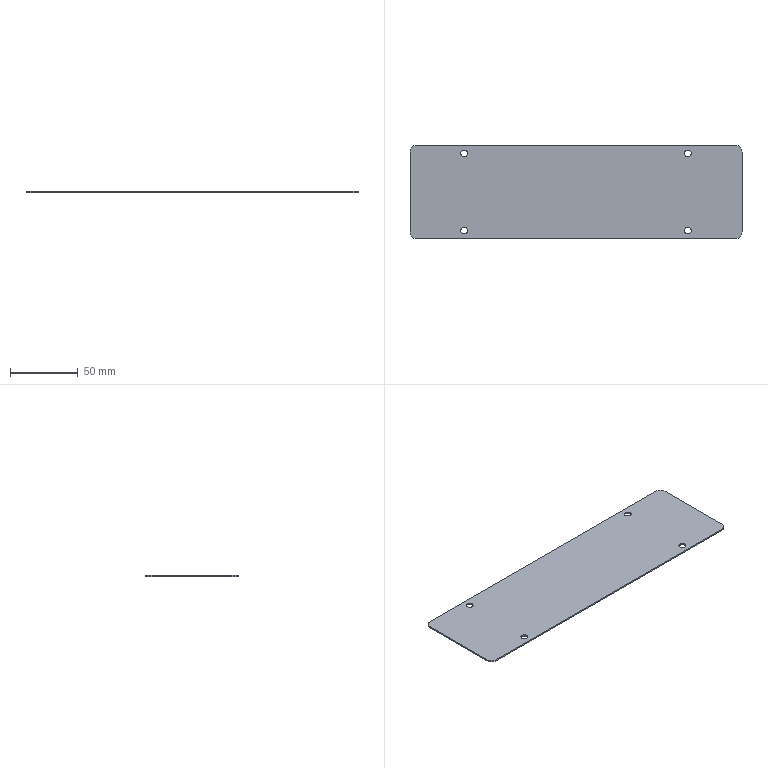Part | SolidWorks | features BaseBody 1 | 1 solid | 18 faces | box 245 x 69 x 1 mm | volume 16805 mm3 | cylinder 12 | plane 6 | commonest cylinder face diameters 5 x8 10 x4
STEP:
#1=CARTESIAN_POINT('',(-85.,-28.5,1.));
#2=VERTEX_POINT('',#1);
#3=CARTESIAN_POINT('',(-80.,-28.5,1.));
#4=VERTEX_POINT('',#3);
#5=CARTESIAN_POINT('',(-82.5,-28.5,1.));
#6=DIRECTION('',(0.,0.,1.));
#7=DIRECTION('',(-1.,0.,0.));
#8=AXIS2_PLACEMENT_3D('',#5,#6,#7);
#9=CIRCLE('',#8,2.5);
#10=EDGE_CURVE('',#2,#4,#9,.T.);
#11=ORIENTED_EDGE('',*,*,#10,.T.);
#12=CARTESIAN_POINT('',(-80.,-28.5,0.));
#13=VERTEX_POINT('',#12);
#14=CARTESIAN_POINT('',(-80.,-28.5,1.));
#15=DIRECTION('',(0.,0.,-1.));
#16=VECTOR('',#15,1000.);
#17=LINE('',#14,#16);
#18=EDGE_CURVE('',#4,#13,#17,.T.);
#19=ORIENTED_EDGE('',*,*,#18,.T.);
#20=CARTESIAN_POINT('',(-85.,-28.5,0.));
#21=VERTEX_POINT('',#20);
#22=CARTESIAN_POINT('',(-82.5,-28.5,0.));
#23=DIRECTION('',(0.,0.,1.));
#24=DIRECTION('',(-1.,0.,0.));
#25=AXIS2_PLACEMENT_3D('',#22,#23,#24);
#26=CIRCLE('',#25,2.5);
#27=EDGE_CURVE('',#21,#13,#26,.T.);
#28=ORIENTED_EDGE('',*,*,#27,.F.);
#29=CARTESIAN_POINT('',(-85.,-28.5,1.));
#30=DIRECTION('',(0.,0.,-1.));
#31=VECTOR('',#30,1000.);
#32=LINE('',#29,#31);
#33=EDGE_CURVE('',#2,#21,#32,.T.);
#34=ORIENTED_EDGE('',*,*,#33,.F.);
#35=EDGE_LOOP('',(#11,#19,#28,#34));
#36=FACE_OUTER_BOUND('',#35,.T.);
#37=CARTESIAN_POINT('',(-82.5,-28.5,1.));
#38=DIRECTION('',(0.,0.,-1.));
#39=DIRECTION('',(-1.,0.,0.));
#40=AXIS2_PLACEMENT_3D('',#37,#38,#39);
#41=CYLINDRICAL_SURFACE('',#40,2.5);
#42=ADVANCED_FACE('',(#36),#41,.F.);
#43=CARTESIAN_POINT('',(80.,-28.5,1.));
#44=VERTEX_POINT('',#43);
#45=CARTESIAN_POINT('',(85.,-28.5,1.));
#46=VERTEX_POINT('',#45);
#47=CARTESIAN_POINT('',(82.5,-28.5,1.));
#48=DIRECTION('',(0.,0.,1.));
#49=DIRECTION('',(-1.,0.,0.));
#50=AXIS2_PLACEMENT_3D('',#47,#48,#49);
#51=CIRCLE('',#50,2.5);
#52=EDGE_CURVE('',#44,#46,#51,.T.);
#53=ORIENTED_EDGE('',*,*,#52,.T.);
#54=CARTESIAN_POINT('',(85.,-28.5,0.));
#55=VERTEX_POINT('',#54);
#56=CARTESIAN_POINT('',(85.,-28.5,1.));
#57=DIRECTION('',(0.,0.,-1.));
#58=VECTOR('',#57,1000.);
#59=LINE('',#56,#58);
#60=EDGE_CURVE('',#46,#55,#59,.T.);
#61=ORIENTED_EDGE('',*,*,#60,.T.);
#62=CARTESIAN_POINT('',(80.,-28.5,0.));
#63=VERTEX_POINT('',#62);
#64=CARTESIAN_POINT('',(82.5,-28.5,0.));
#65=DIRECTION('',(0.,0.,1.));
#66=DIRECTION('',(-1.,0.,0.));
#67=AXIS2_PLACEMENT_3D('',#64,#65,#66);
#68=CIRCLE('',#67,2.5);
#69=EDGE_CURVE('',#63,#55,#68,.T.);
#70=ORIENTED_EDGE('',*,*,#69,.F.);
#71=CARTESIAN_POINT('',(80.,-28.5,1.));
#72=DIRECTION('',(0.,0.,-1.));
#73=VECTOR('',#72,1000.);
#74=LINE('',#71,#73);
#75=EDGE_CURVE('',#44,#63,#74,.T.);
#76=ORIENTED_EDGE('',*,*,#75,.F.);
#77=EDGE_LOOP('',(#53,#61,#70,#76));
#78=FACE_OUTER_BOUND('',#77,.T.);
#79=CARTESIAN_POINT('',(82.5,-28.5,1.));
#80=DIRECTION('',(0.,0.,-1.));
#81=DIRECTION('',(-1.,0.,0.));
#82=AXIS2_PLACEMENT_3D('',#79,#80,#81);
#83=CYLINDRICAL_SURFACE('',#82,2.5);
#84=ADVANCED_FACE('',(#78),#83,.F.);
#85=CARTESIAN_POINT('',(80.,28.5,1.));
#86=VERTEX_POINT('',#85);
#87=CARTESIAN_POINT('',(85.,28.5,1.));
#88=VERTEX_POINT('',#87);
#89=CARTESIAN_POINT('',(82.5,28.5,1.));
#90=DIRECTION('',(0.,0.,1.));
#91=DIRECTION('',(-1.,0.,0.));
#92=AXIS2_PLACEMENT_3D('',#89,#90,#91);
#93=CIRCLE('',#92,2.5);
#94=EDGE_CURVE('',#86,#88,#93,.T.);
#95=ORIENTED_EDGE('',*,*,#94,.T.);
#96=CARTESIAN_POINT('',(85.,28.5,0.));
#97=VERTEX_POINT('',#96);
#98=CARTESIAN_POINT('',(85.,28.5,1.));
#99=DIRECTION('',(0.,0.,-1.));
#100=VECTOR('',#99,1000.);
#101=LINE('',#98,#100);
#102=EDGE_CURVE('',#88,#97,#101,.T.);
#103=ORIENTED_EDGE('',*,*,#102,.T.);
#104=CARTESIAN_POINT('',(80.,28.5,0.));
#105=VERTEX_POINT('',#104);
#106=CARTESIAN_POINT('',(82.5,28.5,0.));
#107=DIRECTION('',(0.,0.,1.));
#108=DIRECTION('',(-1.,0.,0.));
#109=AXIS2_PLACEMENT_3D('',#106,#107,#108);
#110=CIRCLE('',#109,2.5);
#111=EDGE_CURVE('',#105,#97,#110,.T.);
#112=ORIENTED_EDGE('',*,*,#111,.F.);
#113=CARTESIAN_POINT('',(80.,28.5,1.));
#114=DIRECTION('',(0.,0.,-1.));
#115=VECTOR('',#114,1000.);
#116=LINE('',#113,#115);
#117=EDGE_CURVE('',#86,#105,#116,.T.);
#118=ORIENTED_EDGE('',*,*,#117,.F.);
#119=EDGE_LOOP('',(#95,#103,#112,#118));
#120=FACE_OUTER_BOUND('',#119,.T.);
#121=CARTESIAN_POINT('',(82.5,28.5,1.));
#122=DIRECTION('',(0.,0.,-1.));
#123=DIRECTION('',(-1.,0.,0.));
#124=AXIS2_PLACEMENT_3D('',#121,#122,#123);
#125=CYLINDRICAL_SURFACE('',#124,2.5);
#126=ADVANCED_FACE('',(#120),#125,.F.);
#127=CARTESIAN_POINT('',(-85.,28.5,1.));
#128=VERTEX_POINT('',#127);
#129=CARTESIAN_POINT('',(-80.,28.5,1.));
#130=VERTEX_POINT('',#129);
#131=CARTESIAN_POINT('',(-82.5,28.5,1.));
#132=DIRECTION('',(0.,0.,1.));
#133=DIRECTION('',(-1.,0.,0.));
#134=AXIS2_PLACEMENT_3D('',#131,#132,#133);
#135=CIRCLE('',#134,2.5);
#136=EDGE_CURVE('',#128,#130,#135,.T.);
#137=ORIENTED_EDGE('',*,*,#136,.T.);
#138=CARTESIAN_POINT('',(-80.,28.5,0.));
#139=VERTEX_POINT('',#138);
#140=CARTESIAN_POINT('',(-80.,28.5,1.));
#141=DIRECTION('',(0.,0.,-1.));
#142=VECTOR('',#141,1000.);
#143=LINE('',#140,#142);
#144=EDGE_CURVE('',#130,#139,#143,.T.);
#145=ORIENTED_EDGE('',*,*,#144,.T.);
#146=CARTESIAN_POINT('',(-85.,28.5,0.));
#147=VERTEX_POINT('',#146);
#148=CARTESIAN_POINT('',(-82.5,28.5,0.));
#149=DIRECTION('',(0.,0.,1.));
#150=DIRECTION('',(-1.,0.,0.));
#151=AXIS2_PLACEMENT_3D('',#148,#149,#150);
#152=CIRCLE('',#151,2.5);
#153=EDGE_CURVE('',#147,#139,#152,.T.);
#154=ORIENTED_EDGE('',*,*,#153,.F.);
#155=CARTESIAN_POINT('',(-85.,28.5,1.));
#156=DIRECTION('',(0.,0.,-1.));
#157=VECTOR('',#156,1000.);
#158=LINE('',#155,#157);
#159=EDGE_CURVE('',#128,#147,#158,.T.);
#160=ORIENTED_EDGE('',*,*,#159,.F.);
#161=EDGE_LOOP('',(#137,#145,#154,#160));
#162=FACE_OUTER_BOUND('',#161,.T.);
#163=CARTESIAN_POINT('',(-82.5,28.5,1.));
#164=DIRECTION('',(0.,0.,-1.));
#165=DIRECTION('',(-1.,0.,0.));
#166=AXIS2_PLACEMENT_3D('',#163,#164,#165);
#167=CYLINDRICAL_SURFACE('',#166,2.5);
#168=ADVANCED_FACE('',(#162),#167,.F.);
#169=ORIENTED_EDGE('',*,*,#10,.F.);
#170=CARTESIAN_POINT('',(-82.5,-28.5,1.));
#171=DIRECTION('',(0.,0.,1.));
#172=DIRECTION('',(-1.,0.,0.));
#173=AXIS2_PLACEMENT_3D('',#170,#171,#172);
#174=CIRCLE('',#173,2.5);
#175=EDGE_CURVE('',#4,#2,#174,.T.);
#176=ORIENTED_EDGE('',*,*,#175,.F.);
#177=EDGE_LOOP('',(#169,#176));
#178=FACE_BOUND('',#177,.T.);
#179=ORIENTED_EDGE('',*,*,#52,.F.);
#180=CARTESIAN_POINT('',(82.5,-28.5,1.));
#181=DIRECTION('',(0.,0.,1.));
#182=DIRECTION('',(-1.,0.,0.));
#183=AXIS2_PLACEMENT_3D('',#180,#181,#182);
#184=CIRCLE('',#183,2.5);
#185=EDGE_CURVE('',#46,#44,#184,.T.);
#186=ORIENTED_EDGE('',*,*,#185,.F.);
#187=EDGE_LOOP('',(#179,#186));
#188=FACE_BOUND('',#187,.T.);
#189=ORIENTED_EDGE('',*,*,#94,.F.);
#190=CARTESIAN_POINT('',(82.5,28.5,1.));
#191=DIRECTION('',(0.,0.,1.));
#192=DIRECTION('',(-1.,0.,0.));
#193=AXIS2_PLACEMENT_3D('',#190,#191,#192);
#194=CIRCLE('',#193,2.5);
#195=EDGE_CURVE('',#88,#86,#194,.T.);
#196=ORIENTED_EDGE('',*,*,#195,.F.);
#197=EDGE_LOOP('',(#189,#196));
#198=FACE_BOUND('',#197,.T.);
#199=ORIENTED_EDGE('',*,*,#136,.F.);
#200=CARTESIAN_POINT('',(-82.5,28.5,1.));
#201=DIRECTION('',(0.,0.,1.));
#202=DIRECTION('',(-1.,0.,0.));
#203=AXIS2_PLACEMENT_3D('',#200,#201,#202);
#204=CIRCLE('',#203,2.5);
#205=EDGE_CURVE('',#130,#128,#204,.T.);
#206=ORIENTED_EDGE('',*,*,#205,.F.);
#207=EDGE_LOOP('',(#199,#206));
#208=FACE_BOUND('',#207,.T.);
#209=CARTESIAN_POINT('',(117.5,-34.5,1.));
#210=VERTEX_POINT('',#209);
#211=CARTESIAN_POINT('',(-117.5,-34.5,1.));
#212=VERTEX_POINT('',#211);
#213=CARTESIAN_POINT('',(-117.5,-34.5,1.));
#214=DIRECTION('',(-1.,0.,0.));
#215=VECTOR('',#214,1000.);
#216=LINE('',#213,#215);
#217=EDGE_CURVE('',#210,#212,#216,.T.);
#218=ORIENTED_EDGE('',*,*,#217,.F.);
#219=CARTESIAN_POINT('',(122.5,-29.5,1.));
#220=VERTEX_POINT('',#219);
#221=CARTESIAN_POINT('',(117.5,-29.5,1.));
#222=DIRECTION('',(0.,0.,-1.));
#223=DIRECTION('',(-1.,0.,0.));
#224=AXIS2_PLACEMENT_3D('',#221,#222,#223);
#225=CIRCLE('',#224,5.);
#226=EDGE_CURVE('',#220,#210,#225,.T.);
#227=ORIENTED_EDGE('',*,*,#226,.F.);
#228=CARTESIAN_POINT('',(122.5,29.5,1.));
#229=VERTEX_POINT('',#228);
#230=CARTESIAN_POINT('',(122.5,-29.5,1.));
#231=DIRECTION('',(0.,-1.,0.));
#232=VECTOR('',#231,1000.);
#233=LINE('',#230,#232);
#234=EDGE_CURVE('',#229,#220,#233,.T.);
#235=ORIENTED_EDGE('',*,*,#234,.F.);
#236=CARTESIAN_POINT('',(117.5,34.5,1.));
#237=VERTEX_POINT('',#236);
#238=CARTESIAN_POINT('',(117.5,29.5,1.));
#239=DIRECTION('',(0.,0.,-1.));
#240=DIRECTION('',(-1.,0.,0.));
#241=AXIS2_PLACEMENT_3D('',#238,#239,#240);
#242=CIRCLE('',#241,5.);
#243=EDGE_CURVE('',#237,#229,#242,.T.);
#244=ORIENTED_EDGE('',*,*,#243,.F.);
#245=CARTESIAN_POINT('',(-117.5,34.5,1.));
#246=VERTEX_POINT('',#245);
#247=CARTESIAN_POINT('',(-117.5,34.5,1.));
#248=DIRECTION('',(1.,0.,0.));
#249=VECTOR('',#248,1000.);
#250=LINE('',#247,#249);
#251=EDGE_CURVE('',#246,#237,#250,.T.);
#252=ORIENTED_EDGE('',*,*,#251,.F.);
#253=CARTESIAN_POINT('',(-122.5,29.5,1.));
#254=VERTEX_POINT('',#253);
#255=CARTESIAN_POINT('',(-117.5,29.5,1.));
#256=DIRECTION('',(0.,0.,-1.));
#257=DIRECTION('',(-1.,0.,0.));
#258=AXIS2_PLACEMENT_3D('',#255,#256,#257);
#259=CIRCLE('',#258,5.);
#260=EDGE_CURVE('',#254,#246,#259,.T.);
#261=ORIENTED_EDGE('',*,*,#260,.F.);
#262=CARTESIAN_POINT('',(-122.5,-29.5,1.));
#263=VERTEX_POINT('',#262);
#264=CARTESIAN_POINT('',(-122.5,-29.5,1.));
#265=DIRECTION('',(0.,1.,0.));
#266=VECTOR('',#265,1000.);
#267=LINE('',#264,#266);
#268=EDGE_CURVE('',#263,#254,#267,.T.);
#269=ORIENTED_EDGE('',*,*,#268,.F.);
#270=CARTESIAN_POINT('',(-117.5,-29.5,1.));
#271=DIRECTION('',(0.,0.,-1.));
#272=DIRECTION('',(-1.,0.,0.));
#273=AXIS2_PLACEMENT_3D('',#270,#271,#272);
#274=CIRCLE('',#273,5.);
#275=EDGE_CURVE('',#212,#263,#274,.T.);
#276=ORIENTED_EDGE('',*,*,#275,.F.);
#277=EDGE_LOOP('',(#218,#227,#235,#244,#252,#261,#269,#276));
#278=FACE_OUTER_BOUND('',#277,.T.);
#279=CARTESIAN_POINT('',(-117.5,-29.5,1.));
#280=DIRECTION('',(0.,0.,-1.));
#281=DIRECTION('',(-1.,0.,0.));
#282=AXIS2_PLACEMENT_3D('',#279,#280,#281);
#283=PLANE('',#282);
#284=ADVANCED_FACE('',(#178,#188,#198,#208,#278),#283,.F.);
#285=ORIENTED_EDGE('',*,*,#18,.F.);
#286=ORIENTED_EDGE('',*,*,#175,.T.);
#287=ORIENTED_EDGE('',*,*,#33,.T.);
#288=CARTESIAN_POINT('',(-82.5,-28.5,0.));
#289=DIRECTION('',(0.,0.,1.));
#290=DIRECTION('',(-1.,0.,0.));
#291=AXIS2_PLACEMENT_3D('',#288,#289,#290);
#292=CIRCLE('',#291,2.5);
#293=EDGE_CURVE('',#13,#21,#292,.T.);
#294=ORIENTED_EDGE('',*,*,#293,.F.);
#295=EDGE_LOOP('',(#285,#286,#287,#294));
#296=FACE_OUTER_BOUND('',#295,.T.);
#297=CARTESIAN_POINT('',(-82.5,-28.5,1.));
#298=DIRECTION('',(0.,0.,-1.));
#299=DIRECTION('',(-1.,0.,0.));
#300=AXIS2_PLACEMENT_3D('',#297,#298,#299);
#301=CYLINDRICAL_SURFACE('',#300,2.5);
#302=ADVANCED_FACE('',(#296),#301,.F.);
#303=ORIENTED_EDGE('',*,*,#60,.F.);
#304=ORIENTED_EDGE('',*,*,#185,.T.);
#305=ORIENTED_EDGE('',*,*,#75,.T.);
#306=CARTESIAN_POINT('',(82.5,-28.5,0.));
#307=DIRECTION('',(0.,0.,1.));
#308=DIRECTION('',(-1.,0.,0.));
#309=AXIS2_PLACEMENT_3D('',#306,#307,#308);
#310=CIRCLE('',#309,2.5);
#311=EDGE_CURVE('',#55,#63,#310,.T.);
#312=ORIENTED_EDGE('',*,*,#311,.F.);
#313=EDGE_LOOP('',(#303,#304,#305,#312));
#314=FACE_OUTER_BOUND('',#313,.T.);
#315=CARTESIAN_POINT('',(82.5,-28.5,1.));
#316=DIRECTION('',(0.,0.,-1.));
#317=DIRECTION('',(-1.,0.,0.));
#318=AXIS2_PLACEMENT_3D('',#315,#316,#317);
#319=CYLINDRICAL_SURFACE('',#318,2.5);
#320=ADVANCED_FACE('',(#314),#319,.F.);
#321=ORIENTED_EDGE('',*,*,#102,.F.);
#322=ORIENTED_EDGE('',*,*,#195,.T.);
#323=ORIENTED_EDGE('',*,*,#117,.T.);
#324=CARTESIAN_POINT('',(82.5,28.5,0.));
#325=DIRECTION('',(0.,0.,1.));
#326=DIRECTION('',(-1.,0.,0.));
#327=AXIS2_PLACEMENT_3D('',#324,#325,#326);
#328=CIRCLE('',#327,2.5);
#329=EDGE_CURVE('',#97,#105,#328,.T.);
#330=ORIENTED_EDGE('',*,*,#329,.F.);
#331=EDGE_LOOP('',(#321,#322,#323,#330));
#332=FACE_OUTER_BOUND('',#331,.T.);
#333=CARTESIAN_POINT('',(82.5,28.5,1.));
#334=DIRECTION('',(0.,0.,-1.));
#335=DIRECTION('',(-1.,0.,0.));
#336=AXIS2_PLACEMENT_3D('',#333,#334,#335);
#337=CYLINDRICAL_SURFACE('',#336,2.5);
#338=ADVANCED_FACE('',(#332),#337,.F.);
#339=ORIENTED_EDGE('',*,*,#144,.F.);
#340=ORIENTED_EDGE('',*,*,#205,.T.);
#341=ORIENTED_EDGE('',*,*,#159,.T.);
#342=CARTESIAN_POINT('',(-82.5,28.5,0.));
#343=DIRECTION('',(0.,0.,1.));
#344=DIRECTION('',(-1.,0.,0.));
#345=AXIS2_PLACEMENT_3D('',#342,#343,#344);
#346=CIRCLE('',#345,2.5);
#347=EDGE_CURVE('',#139,#147,#346,.T.);
#348=ORIENTED_EDGE('',*,*,#347,.F.);
#349=EDGE_LOOP('',(#339,#340,#341,#348));
#350=FACE_OUTER_BOUND('',#349,.T.);
#351=CARTESIAN_POINT('',(-82.5,28.5,1.));
#352=DIRECTION('',(0.,0.,-1.));
#353=DIRECTION('',(-1.,0.,0.));
#354=AXIS2_PLACEMENT_3D('',#351,#352,#353);
#355=CYLINDRICAL_SURFACE('',#354,2.5);
#356=ADVANCED_FACE('',(#350),#355,.F.);
#357=ORIENTED_EDGE('',*,*,#275,.T.);
#358=CARTESIAN_POINT('',(-122.5,-29.5,0.));
#359=VERTEX_POINT('',#358);
#360=CARTESIAN_POINT('',(-122.5,-29.5,1.));
#361=DIRECTION('',(0.,0.,-1.));
#362=VECTOR('',#361,1000.);
#363=LINE('',#360,#362);
#364=EDGE_CURVE('',#263,#359,#363,.T.);
#365=ORIENTED_EDGE('',*,*,#364,.T.);
#366=CARTESIAN_POINT('',(-117.5,-34.5,0.));
#367=VERTEX_POINT('',#366);
#368=CARTESIAN_POINT('',(-117.5,-29.5,0.));
#369=DIRECTION('',(0.,0.,1.));
#370=DIRECTION('',(-1.,0.,0.));
#371=AXIS2_PLACEMENT_3D('',#368,#369,#370);
#372=CIRCLE('',#371,5.);
#373=EDGE_CURVE('',#359,#367,#372,.T.);
#374=ORIENTED_EDGE('',*,*,#373,.T.);
#375=CARTESIAN_POINT('',(-117.5,-34.5,1.));
#376=DIRECTION('',(0.,0.,1.));
#377=VECTOR('',#376,1000.);
#378=LINE('',#375,#377);
#379=EDGE_CURVE('',#367,#212,#378,.T.);
#380=ORIENTED_EDGE('',*,*,#379,.T.);
#381=EDGE_LOOP('',(#357,#365,#374,#380));
#382=FACE_OUTER_BOUND('',#381,.T.);
#383=CARTESIAN_POINT('',(-117.5,-29.5,1.));
#384=DIRECTION('',(0.,0.,-1.));
#385=DIRECTION('',(-1.,0.,0.));
#386=AXIS2_PLACEMENT_3D('',#383,#384,#385);
#387=CYLINDRICAL_SURFACE('',#386,5.);
#388=ADVANCED_FACE('',(#382),#387,.T.);
#389=CARTESIAN_POINT('',(117.5,-34.5,0.));
#390=VERTEX_POINT('',#389);
#391=CARTESIAN_POINT('',(117.5,-34.5,1.));
#392=DIRECTION('',(0.,0.,-1.));
#393=VECTOR('',#392,1000.);
#394=LINE('',#391,#393);
#395=EDGE_CURVE('',#210,#390,#394,.T.);
#396=ORIENTED_EDGE('',*,*,#395,.F.);
#397=ORIENTED_EDGE('',*,*,#217,.T.);
#398=ORIENTED_EDGE('',*,*,#379,.F.);
#399=CARTESIAN_POINT('',(117.5,-34.5,0.));
#400=DIRECTION('',(-1.,0.,0.));
#401=VECTOR('',#400,1000.);
#402=LINE('',#399,#401);
#403=EDGE_CURVE('',#390,#367,#402,.T.);
#404=ORIENTED_EDGE('',*,*,#403,.F.);
#405=EDGE_LOOP('',(#396,#397,#398,#404));
#406=FACE_OUTER_BOUND('',#405,.T.);
#407=CARTESIAN_POINT('',(117.5,-34.5,1.));
#408=DIRECTION('',(0.,1.,0.));
#409=DIRECTION('',(-1.,0.,0.));
#410=AXIS2_PLACEMENT_3D('',#407,#408,#409);
#411=PLANE('',#410);
#412=ADVANCED_FACE('',(#406),#411,.F.);
#413=ORIENTED_EDGE('',*,*,#226,.T.);
#414=ORIENTED_EDGE('',*,*,#395,.T.);
#415=CARTESIAN_POINT('',(122.5,-29.5,0.));
#416=VERTEX_POINT('',#415);
#417=CARTESIAN_POINT('',(117.5,-29.5,0.));
#418=DIRECTION('',(0.,0.,1.));
#419=DIRECTION('',(-1.,0.,0.));
#420=AXIS2_PLACEMENT_3D('',#417,#418,#419);
#421=CIRCLE('',#420,5.);
#422=EDGE_CURVE('',#390,#416,#421,.T.);
#423=ORIENTED_EDGE('',*,*,#422,.T.);
#424=CARTESIAN_POINT('',(122.5,-29.5,1.));
#425=DIRECTION('',(0.,0.,1.));
#426=VECTOR('',#425,1000.);
#427=LINE('',#424,#426);
#428=EDGE_CURVE('',#416,#220,#427,.T.);
#429=ORIENTED_EDGE('',*,*,#428,.T.);
#430=EDGE_LOOP('',(#413,#414,#423,#429));
#431=FACE_OUTER_BOUND('',#430,.T.);
#432=CARTESIAN_POINT('',(117.5,-29.5,1.));
#433=DIRECTION('',(0.,0.,-1.));
#434=DIRECTION('',(-1.,0.,0.));
#435=AXIS2_PLACEMENT_3D('',#432,#433,#434);
#436=CYLINDRICAL_SURFACE('',#435,5.);
#437=ADVANCED_FACE('',(#431),#436,.T.);
#438=CARTESIAN_POINT('',(122.5,29.5,0.));
#439=VERTEX_POINT('',#438);
#440=CARTESIAN_POINT('',(122.5,29.5,1.));
#441=DIRECTION('',(0.,0.,-1.));
#442=VECTOR('',#441,1000.);
#443=LINE('',#440,#442);
#444=EDGE_CURVE('',#229,#439,#443,.T.);
#445=ORIENTED_EDGE('',*,*,#444,.F.);
#446=ORIENTED_EDGE('',*,*,#234,.T.);
#447=ORIENTED_EDGE('',*,*,#428,.F.);
#448=CARTESIAN_POINT('',(122.5,29.5,0.));
#449=DIRECTION('',(0.,-1.,0.));
#450=VECTOR('',#449,1000.);
#451=LINE('',#448,#450);
#452=EDGE_CURVE('',#439,#416,#451,.T.);
#453=ORIENTED_EDGE('',*,*,#452,.F.);
#454=EDGE_LOOP('',(#445,#446,#447,#453));
#455=FACE_OUTER_BOUND('',#454,.T.);
#456=CARTESIAN_POINT('',(122.5,29.5,1.));
#457=DIRECTION('',(-1.,0.,0.));
#458=DIRECTION('',(0.,-1.,0.));
#459=AXIS2_PLACEMENT_3D('',#456,#457,#458);
#460=PLANE('',#459);
#461=ADVANCED_FACE('',(#455),#460,.F.);
#462=ORIENTED_EDGE('',*,*,#243,.T.);
#463=ORIENTED_EDGE('',*,*,#444,.T.);
#464=CARTESIAN_POINT('',(117.5,34.5,0.));
#465=VERTEX_POINT('',#464);
#466=CARTESIAN_POINT('',(117.5,29.5,0.));
#467=DIRECTION('',(0.,0.,1.));
#468=DIRECTION('',(-1.,0.,0.));
#469=AXIS2_PLACEMENT_3D('',#466,#467,#468);
#470=CIRCLE('',#469,5.);
#471=EDGE_CURVE('',#439,#465,#470,.T.);
#472=ORIENTED_EDGE('',*,*,#471,.T.);
#473=CARTESIAN_POINT('',(117.5,34.5,1.));
#474=DIRECTION('',(0.,0.,1.));
#475=VECTOR('',#474,1000.);
#476=LINE('',#473,#475);
#477=EDGE_CURVE('',#465,#237,#476,.T.);
#478=ORIENTED_EDGE('',*,*,#477,.T.);
#479=EDGE_LOOP('',(#462,#463,#472,#478));
#480=FACE_OUTER_BOUND('',#479,.T.);
#481=CARTESIAN_POINT('',(117.5,29.5,1.));
#482=DIRECTION('',(0.,0.,-1.));
#483=DIRECTION('',(-1.,0.,0.));
#484=AXIS2_PLACEMENT_3D('',#481,#482,#483);
#485=CYLINDRICAL_SURFACE('',#484,5.);
#486=ADVANCED_FACE('',(#480),#485,.T.);
#487=CARTESIAN_POINT('',(-117.5,34.5,0.));
#488=VERTEX_POINT('',#487);
#489=CARTESIAN_POINT('',(-117.5,34.5,1.));
#490=DIRECTION('',(0.,0.,-1.));
#491=VECTOR('',#490,1000.);
#492=LINE('',#489,#491);
#493=EDGE_CURVE('',#246,#488,#492,.T.);
#494=ORIENTED_EDGE('',*,*,#493,.F.);
#495=ORIENTED_EDGE('',*,*,#251,.T.);
#496=ORIENTED_EDGE('',*,*,#477,.F.);
#497=CARTESIAN_POINT('',(117.5,34.5,0.));
#498=DIRECTION('',(1.,0.,0.));
#499=VECTOR('',#498,1000.);
#500=LINE('',#497,#499);
#501=EDGE_CURVE('',#488,#465,#500,.T.);
#502=ORIENTED_EDGE('',*,*,#501,.F.);
#503=EDGE_LOOP('',(#494,#495,#496,#502));
#504=FACE_OUTER_BOUND('',#503,.T.);
#505=CARTESIAN_POINT('',(117.5,34.5,1.));
#506=DIRECTION('',(0.,-1.,0.));
#507=DIRECTION('',(1.,0.,0.));
#508=AXIS2_PLACEMENT_3D('',#505,#506,#507);
#509=PLANE('',#508);
#510=ADVANCED_FACE('',(#504),#509,.F.);
#511=ORIENTED_EDGE('',*,*,#260,.T.);
#512=ORIENTED_EDGE('',*,*,#493,.T.);
#513=CARTESIAN_POINT('',(-122.5,29.5,0.));
#514=VERTEX_POINT('',#513);
#515=CARTESIAN_POINT('',(-117.5,29.5,0.));
#516=DIRECTION('',(0.,0.,1.));
#517=DIRECTION('',(-1.,0.,0.));
#518=AXIS2_PLACEMENT_3D('',#515,#516,#517);
#519=CIRCLE('',#518,5.);
#520=EDGE_CURVE('',#488,#514,#519,.T.);
#521=ORIENTED_EDGE('',*,*,#520,.T.);
#522=CARTESIAN_POINT('',(-122.5,29.5,1.));
#523=DIRECTION('',(0.,0.,1.));
#524=VECTOR('',#523,1000.);
#525=LINE('',#522,#524);
#526=EDGE_CURVE('',#514,#254,#525,.T.);
#527=ORIENTED_EDGE('',*,*,#526,.T.);
#528=EDGE_LOOP('',(#511,#512,#521,#527));
#529=FACE_OUTER_BOUND('',#528,.T.);
#530=CARTESIAN_POINT('',(-117.5,29.5,1.));
#531=DIRECTION('',(0.,0.,-1.));
#532=DIRECTION('',(-1.,0.,0.));
#533=AXIS2_PLACEMENT_3D('',#530,#531,#532);
#534=CYLINDRICAL_SURFACE('',#533,5.);
#535=ADVANCED_FACE('',(#529),#534,.T.);
#536=ORIENTED_EDGE('',*,*,#364,.F.);
#537=ORIENTED_EDGE('',*,*,#268,.T.);
#538=ORIENTED_EDGE('',*,*,#526,.F.);
#539=CARTESIAN_POINT('',(-122.5,29.5,0.));
#540=DIRECTION('',(0.,1.,0.));
#541=VECTOR('',#540,1000.);
#542=LINE('',#539,#541);
#543=EDGE_CURVE('',#359,#514,#542,.T.);
#544=ORIENTED_EDGE('',*,*,#543,.F.);
#545=EDGE_LOOP('',(#536,#537,#538,#544));
#546=FACE_OUTER_BOUND('',#545,.T.);
#547=CARTESIAN_POINT('',(-122.5,29.5,1.));
#548=DIRECTION('',(1.,0.,0.));
#549=DIRECTION('',(0.,1.,0.));
#550=AXIS2_PLACEMENT_3D('',#547,#548,#549);
#551=PLANE('',#550);
#552=ADVANCED_FACE('',(#546),#551,.F.);
#553=ORIENTED_EDGE('',*,*,#27,.T.);
#554=ORIENTED_EDGE('',*,*,#293,.T.);
#555=EDGE_LOOP('',(#553,#554));
#556=FACE_BOUND('',#555,.T.);
#557=ORIENTED_EDGE('',*,*,#111,.T.);
#558=ORIENTED_EDGE('',*,*,#329,.T.);
#559=EDGE_LOOP('',(#557,#558));
#560=FACE_BOUND('',#559,.T.);
#561=ORIENTED_EDGE('',*,*,#153,.T.);
#562=ORIENTED_EDGE('',*,*,#347,.T.);
#563=EDGE_LOOP('',(#561,#562));
#564=FACE_BOUND('',#563,.T.);
#565=ORIENTED_EDGE('',*,*,#69,.T.);
#566=ORIENTED_EDGE('',*,*,#311,.T.);
#567=EDGE_LOOP('',(#565,#566));
#568=FACE_BOUND('',#567,.T.);
#569=ORIENTED_EDGE('',*,*,#422,.F.);
#570=ORIENTED_EDGE('',*,*,#403,.T.);
#571=ORIENTED_EDGE('',*,*,#373,.F.);
#572=ORIENTED_EDGE('',*,*,#543,.T.);
#573=ORIENTED_EDGE('',*,*,#520,.F.);
#574=ORIENTED_EDGE('',*,*,#501,.T.);
#575=ORIENTED_EDGE('',*,*,#471,.F.);
#576=ORIENTED_EDGE('',*,*,#452,.T.);
#577=EDGE_LOOP('',(#569,#570,#571,#572,#573,#574,#575,#576));
#578=FACE_OUTER_BOUND('',#577,.T.);
#579=CARTESIAN_POINT('',(-117.5,-29.5,0.));
#580=DIRECTION('',(0.,0.,-1.));
#581=DIRECTION('',(-1.,0.,0.));
#582=AXIS2_PLACEMENT_3D('',#579,#580,#581);
#583=PLANE('',#582);
#584=ADVANCED_FACE('',(#556,#560,#564,#568,#578),#583,.T.);
#585=CLOSED_SHELL('',(#42,#84,#126,#168,#284,#302,#320,#338,#356,#388,#412,#437,#461,#486,#510,#535,#552,#584));
#586=MANIFOLD_SOLID_BREP('',#585);
#587=CARTESIAN_POINT('',(0.,0.,0.));
#588=DIRECTION('',(0.,0.,1.));
#589=DIRECTION('',(1.,0.,0.));
#590=AXIS2_PLACEMENT_3D('',#587,#588,#589);
#591=(LENGTH_UNIT()NAMED_UNIT(*)SI_UNIT(.MILLI.,.METRE.));
#592=UNCERTAINTY_MEASURE_WITH_UNIT(LENGTH_MEASURE(0.00001),#591,'','');
#593=(NAMED_UNIT(*)PLANE_ANGLE_UNIT()SI_UNIT($,.RADIAN.));
#594=(NAMED_UNIT(*)SI_UNIT($,.STERADIAN.)SOLID_ANGLE_UNIT());
#595=(GEOMETRIC_REPRESENTATION_CONTEXT(3)GLOBAL_UNCERTAINTY_ASSIGNED_CONTEXT((#592))GLOBAL_UNIT_ASSIGNED_CONTEXT((#591,#593,#594))REPRESENTATION_CONTEXT('',''));
#596=ADVANCED_BREP_SHAPE_REPRESENTATION('',(#586,#590),#595);